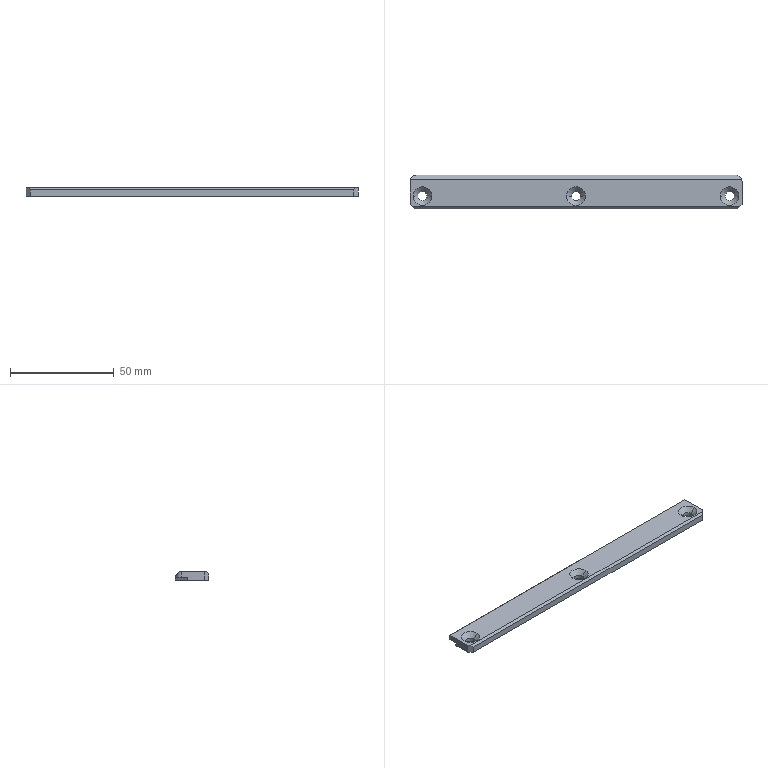Part | STEP file | QA-AD05 | 1 solid | 26 faces | box 160 x 16 x 4 mm | volume 9462 mm3 | plane 12 | cylinder 8 | cone 6 | commonest cylinder face diameters 4.5 x6 6 x2